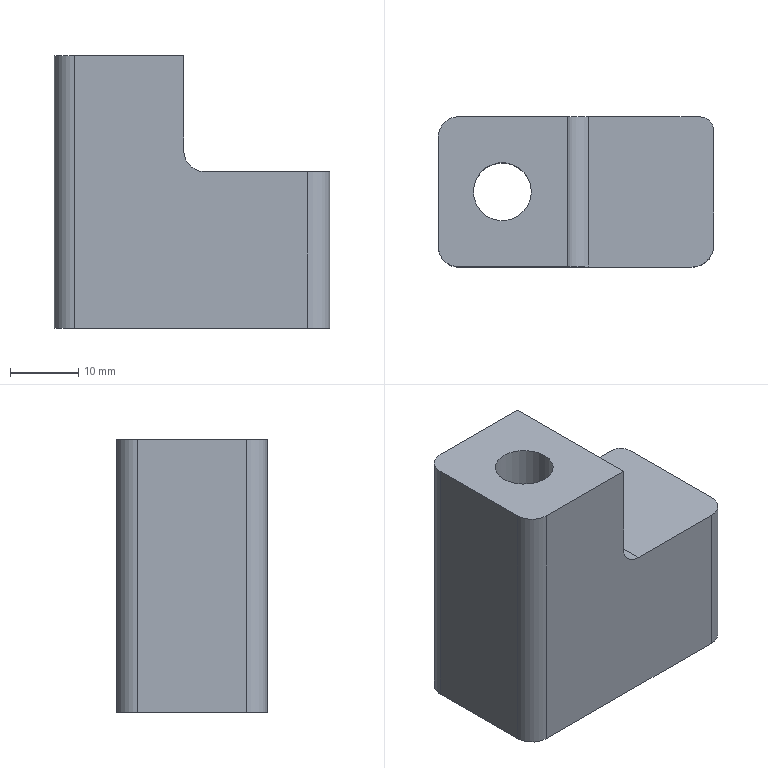Part | NX | features PS-10 2 | 1 solid | 16 faces | box 40.4 x 22 x 40 mm | volume 23471 mm3 | plane 9 | cylinder 7 | commonest cylinder face diameters 6 x3 4 x1 6.4 x1 8.5 x1 14.5 x1
STEP:
#1=CARTESIAN_POINT('',(2525.885,-823.322,883.716));
#2=VERTEX_POINT('',#1);
#3=CARTESIAN_POINT('',(2509.485,-823.322,883.716));
#4=VERTEX_POINT('',#3);
#5=CARTESIAN_POINT('',(-0.000000017,-823.322,883.716));
#6=DIRECTION('',(-1.,0.,0.));
#7=VECTOR('',#6,1000.);
#8=LINE('',#5,#7);
#9=EDGE_CURVE('',#2,#4,#8,.T.);
#10=ORIENTED_EDGE('',*,*,#9,.T.);
#11=CARTESIAN_POINT('',(2509.485,-845.322,883.716));
#12=VERTEX_POINT('',#11);
#13=CARTESIAN_POINT('',(2509.485,0.,883.716));
#14=DIRECTION('',(0.,1.,0.));
#15=VECTOR('',#14,1000.);
#16=LINE('',#13,#15);
#17=EDGE_CURVE('',#4,#12,#16,.F.);
#18=ORIENTED_EDGE('',*,*,#17,.T.);
#19=CARTESIAN_POINT('',(2524.685,-845.322,883.716));
#20=VERTEX_POINT('',#19);
#21=CARTESIAN_POINT('',(0.,-845.322,883.716));
#22=DIRECTION('',(-1.,0.,0.));
#23=VECTOR('',#22,1000.);
#24=LINE('',#21,#23);
#25=EDGE_CURVE('',#20,#12,#24,.T.);
#26=ORIENTED_EDGE('',*,*,#25,.F.);
#27=CARTESIAN_POINT('',(2527.885,-842.122,883.716));
#28=VERTEX_POINT('',#27);
#29=CARTESIAN_POINT('',(2524.685,-842.122,883.716));
#30=DIRECTION('',(0.,0.,1.));
#31=DIRECTION('',(1.,0.,0.));
#32=AXIS2_PLACEMENT_3D('',#29,#30,#31);
#33=CIRCLE('',#32,3.2);
#34=EDGE_CURVE('',#20,#28,#33,.T.);
#35=ORIENTED_EDGE('',*,*,#34,.T.);
#36=CARTESIAN_POINT('',(2527.885,-825.322,883.716));
#37=VERTEX_POINT('',#36);
#38=CARTESIAN_POINT('',(2527.885,0.,883.716));
#39=DIRECTION('',(0.,-1.,0.));
#40=VECTOR('',#39,1000.);
#41=LINE('',#38,#40);
#42=EDGE_CURVE('',#37,#28,#41,.T.);
#43=ORIENTED_EDGE('',*,*,#42,.F.);
#44=CARTESIAN_POINT('',(2525.885,-825.322,883.716));
#45=DIRECTION('',(0.,0.,1.));
#46=DIRECTION('',(1.,0.,0.));
#47=AXIS2_PLACEMENT_3D('',#44,#45,#46);
#48=CIRCLE('',#47,2.);
#49=EDGE_CURVE('',#37,#2,#48,.T.);
#50=ORIENTED_EDGE('',*,*,#49,.T.);
#51=EDGE_LOOP('',(#10,#18,#26,#35,#43,#50));
#52=FACE_BOUND('',#51,.T.);
#53=CARTESIAN_POINT('',(0.,0.,883.716));
#54=DIRECTION('',(0.,0.,1.));
#55=DIRECTION('',(1.,0.,0.));
#56=AXIS2_PLACEMENT_3D('',#53,#54,#55);
#57=PLANE('',#56);
#58=ADVANCED_FACE('',(#52),#57,.T.);
#59=CARTESIAN_POINT('',(2487.485,-842.322,860.716));
#60=VERTEX_POINT('',#59);
#61=CARTESIAN_POINT('',(2487.485,-826.322,860.716));
#62=VERTEX_POINT('',#61);
#63=CARTESIAN_POINT('',(2487.485,0.,860.716));
#64=DIRECTION('',(0.,1.,0.));
#65=VECTOR('',#64,1000.);
#66=LINE('',#63,#65);
#67=EDGE_CURVE('',#60,#62,#66,.T.);
#68=ORIENTED_EDGE('',*,*,#67,.F.);
#69=CARTESIAN_POINT('',(2487.485,-842.322,900.716));
#70=VERTEX_POINT('',#69);
#71=CARTESIAN_POINT('',(2487.485,-842.322,861.517));
#72=DIRECTION('',(0.,0.,1.));
#73=VECTOR('',#72,1000.);
#74=LINE('',#71,#73);
#75=EDGE_CURVE('',#60,#70,#74,.T.);
#76=ORIENTED_EDGE('',*,*,#75,.T.);
#77=CARTESIAN_POINT('',(2487.485,-826.322,900.716));
#78=VERTEX_POINT('',#77);
#79=CARTESIAN_POINT('',(2487.485,-823.072,900.716));
#80=DIRECTION('',(0.,-1.,0.));
#81=VECTOR('',#80,1000.);
#82=LINE('',#79,#81);
#83=EDGE_CURVE('',#78,#70,#82,.T.);
#84=ORIENTED_EDGE('',*,*,#83,.F.);
#85=CARTESIAN_POINT('',(2487.485,-826.322,861.517));
#86=DIRECTION('',(0.,0.,1.));
#87=VECTOR('',#86,1000.);
#88=LINE('',#85,#87);
#89=EDGE_CURVE('',#78,#62,#88,.F.);
#90=ORIENTED_EDGE('',*,*,#89,.T.);
#91=EDGE_LOOP('',(#68,#76,#84,#90));
#92=FACE_BOUND('',#91,.T.);
#93=CARTESIAN_POINT('',(2487.485,-823.072,861.517));
#94=DIRECTION('',(1.,0.,0.));
#95=DIRECTION('',(0.,0.,-1.));
#96=AXIS2_PLACEMENT_3D('',#93,#94,#95);
#97=PLANE('',#96);
#98=ADVANCED_FACE('',(#92),#97,.F.);
#99=ORIENTED_EDGE('',*,*,#25,.T.);
#100=CARTESIAN_POINT('',(2506.485,-845.322,886.716));
#101=VERTEX_POINT('',#100);
#102=CARTESIAN_POINT('',(2509.485,-845.322,886.716));
#103=DIRECTION('',(0.,1.,0.));
#104=DIRECTION('',(0.,0.,1.));
#105=AXIS2_PLACEMENT_3D('',#102,#103,#104);
#106=CIRCLE('',#105,3.);
#107=EDGE_CURVE('',#12,#101,#106,.T.);
#108=ORIENTED_EDGE('',*,*,#107,.T.);
#109=CARTESIAN_POINT('',(2506.485,-845.322,900.716));
#110=VERTEX_POINT('',#109);
#111=CARTESIAN_POINT('',(2506.485,-845.322,900.716));
#112=DIRECTION('',(0.,0.,-1.));
#113=VECTOR('',#112,1000.);
#114=LINE('',#111,#113);
#115=EDGE_CURVE('',#101,#110,#114,.F.);
#116=ORIENTED_EDGE('',*,*,#115,.T.);
#117=CARTESIAN_POINT('',(2490.485,-845.322,900.716));
#118=VERTEX_POINT('',#117);
#119=CARTESIAN_POINT('',(2507.11,-845.322,900.716));
#120=DIRECTION('',(-1.,0.,0.));
#121=VECTOR('',#120,1000.);
#122=LINE('',#119,#121);
#123=EDGE_CURVE('',#110,#118,#122,.T.);
#124=ORIENTED_EDGE('',*,*,#123,.T.);
#125=CARTESIAN_POINT('',(2490.485,-845.322,860.716));
#126=VERTEX_POINT('',#125);
#127=CARTESIAN_POINT('',(2490.485,-845.322,861.517));
#128=DIRECTION('',(0.,0.,1.));
#129=VECTOR('',#128,1000.);
#130=LINE('',#127,#129);
#131=EDGE_CURVE('',#118,#126,#130,.F.);
#132=ORIENTED_EDGE('',*,*,#131,.T.);
#133=CARTESIAN_POINT('',(2524.685,-845.322,860.716));
#134=VERTEX_POINT('',#133);
#135=CARTESIAN_POINT('',(0.,-845.322,860.716));
#136=DIRECTION('',(-1.,0.,0.));
#137=VECTOR('',#136,1000.);
#138=LINE('',#135,#137);
#139=EDGE_CURVE('',#134,#126,#138,.T.);
#140=ORIENTED_EDGE('',*,*,#139,.F.);
#141=CARTESIAN_POINT('',(2524.685,-845.322,861.517));
#142=DIRECTION('',(0.,0.,1.));
#143=VECTOR('',#142,1000.);
#144=LINE('',#141,#143);
#145=EDGE_CURVE('',#134,#20,#144,.T.);
#146=ORIENTED_EDGE('',*,*,#145,.T.);
#147=EDGE_LOOP('',(#99,#108,#116,#124,#132,#140,#146));
#148=FACE_BOUND('',#147,.T.);
#149=CARTESIAN_POINT('',(2507.11,-845.322,861.517));
#150=DIRECTION('',(0.,1.,0.));
#151=DIRECTION('',(0.,0.,1.));
#152=AXIS2_PLACEMENT_3D('',#149,#150,#151);
#153=PLANE('',#152);
#154=ADVANCED_FACE('',(#148),#153,.F.);
#155=ORIENTED_EDGE('',*,*,#34,.F.);
#156=ORIENTED_EDGE('',*,*,#145,.F.);
#157=CARTESIAN_POINT('',(2527.885,-842.122,860.716));
#158=VERTEX_POINT('',#157);
#159=CARTESIAN_POINT('',(2524.685,-842.122,860.716));
#160=DIRECTION('',(0.,0.,1.));
#161=DIRECTION('',(1.,0.,0.));
#162=AXIS2_PLACEMENT_3D('',#159,#160,#161);
#163=CIRCLE('',#162,3.2);
#164=EDGE_CURVE('',#134,#158,#163,.T.);
#165=ORIENTED_EDGE('',*,*,#164,.T.);
#166=CARTESIAN_POINT('',(2527.885,-842.122,861.517));
#167=DIRECTION('',(0.,0.,1.));
#168=VECTOR('',#167,1000.);
#169=LINE('',#166,#168);
#170=EDGE_CURVE('',#158,#28,#169,.T.);
#171=ORIENTED_EDGE('',*,*,#170,.T.);
#172=EDGE_LOOP('',(#155,#156,#165,#171));
#173=FACE_BOUND('',#172,.T.);
#174=CARTESIAN_POINT('',(2524.685,-842.122,861.517));
#175=DIRECTION('',(0.,0.,1.));
#176=DIRECTION('',(1.,0.,0.));
#177=AXIS2_PLACEMENT_3D('',#174,#175,#176);
#178=CYLINDRICAL_SURFACE('',#177,3.2);
#179=ADVANCED_FACE('',(#173),#178,.T.);
#180=CARTESIAN_POINT('',(2527.885,-825.322,860.716));
#181=VERTEX_POINT('',#180);
#182=CARTESIAN_POINT('',(2527.885,0.,860.716));
#183=DIRECTION('',(0.,-1.,0.));
#184=VECTOR('',#183,1000.);
#185=LINE('',#182,#184);
#186=EDGE_CURVE('',#181,#158,#185,.T.);
#187=ORIENTED_EDGE('',*,*,#186,.F.);
#188=CARTESIAN_POINT('',(2527.885,-825.322,872.716));
#189=DIRECTION('',(0.,0.,1.));
#190=VECTOR('',#189,1000.);
#191=LINE('',#188,#190);
#192=EDGE_CURVE('',#181,#37,#191,.T.);
#193=ORIENTED_EDGE('',*,*,#192,.T.);
#194=ORIENTED_EDGE('',*,*,#42,.T.);
#195=ORIENTED_EDGE('',*,*,#170,.F.);
#196=EDGE_LOOP('',(#187,#193,#194,#195));
#197=FACE_BOUND('',#196,.T.);
#198=CARTESIAN_POINT('',(2527.885,-823.122,861.517));
#199=DIRECTION('',(-1.,0.,0.));
#200=DIRECTION('',(0.,0.,1.));
#201=AXIS2_PLACEMENT_3D('',#198,#199,#200);
#202=PLANE('',#201);
#203=ADVANCED_FACE('',(#197),#202,.F.);
#204=ORIENTED_EDGE('',*,*,#9,.F.);
#205=CARTESIAN_POINT('',(2525.885,-823.322,860.716));
#206=VERTEX_POINT('',#205);
#207=CARTESIAN_POINT('',(2525.885,-823.322,860.716));
#208=DIRECTION('',(0.,0.,1.));
#209=VECTOR('',#208,1000.);
#210=LINE('',#207,#209);
#211=EDGE_CURVE('',#2,#206,#210,.F.);
#212=ORIENTED_EDGE('',*,*,#211,.T.);
#213=CARTESIAN_POINT('',(2490.485,-823.322,860.716));
#214=VERTEX_POINT('',#213);
#215=CARTESIAN_POINT('',(-0.000000017,-823.322,860.716));
#216=DIRECTION('',(-1.,0.,0.));
#217=VECTOR('',#216,1000.);
#218=LINE('',#215,#217);
#219=EDGE_CURVE('',#206,#214,#218,.T.);
#220=ORIENTED_EDGE('',*,*,#219,.T.);
#221=CARTESIAN_POINT('',(2490.485,-823.322,900.716));
#222=VERTEX_POINT('',#221);
#223=CARTESIAN_POINT('',(2490.485,-823.322,861.517));
#224=DIRECTION('',(0.,0.,1.));
#225=VECTOR('',#224,1000.);
#226=LINE('',#223,#225);
#227=EDGE_CURVE('',#214,#222,#226,.T.);
#228=ORIENTED_EDGE('',*,*,#227,.T.);
#229=CARTESIAN_POINT('',(2506.485,-823.322,900.716));
#230=VERTEX_POINT('',#229);
#231=CARTESIAN_POINT('',(2656.665,-823.322,900.716));
#232=DIRECTION('',(1.,0.,0.));
#233=VECTOR('',#232,1000.);
#234=LINE('',#231,#233);
#235=EDGE_CURVE('',#222,#230,#234,.T.);
#236=ORIENTED_EDGE('',*,*,#235,.T.);
#237=CARTESIAN_POINT('',(2506.485,-823.322,886.716));
#238=VERTEX_POINT('',#237);
#239=CARTESIAN_POINT('',(2506.485,-823.322,900.716));
#240=DIRECTION('',(0.,0.,-1.));
#241=VECTOR('',#240,1000.);
#242=LINE('',#239,#241);
#243=EDGE_CURVE('',#230,#238,#242,.T.);
#244=ORIENTED_EDGE('',*,*,#243,.T.);
#245=CARTESIAN_POINT('',(2509.485,-823.322,886.716));
#246=DIRECTION('',(0.,1.,0.));
#247=DIRECTION('',(-1.,0.,0.));
#248=AXIS2_PLACEMENT_3D('',#245,#246,#247);
#249=CIRCLE('',#248,3.);
#250=EDGE_CURVE('',#238,#4,#249,.F.);
#251=ORIENTED_EDGE('',*,*,#250,.T.);
#252=EDGE_LOOP('',(#204,#212,#220,#228,#236,#244,#251));
#253=FACE_BOUND('',#252,.T.);
#254=CARTESIAN_POINT('',(2656.665,-823.322,861.517));
#255=DIRECTION('',(0.,1.,0.));
#256=DIRECTION('',(-1.,0.,0.));
#257=AXIS2_PLACEMENT_3D('',#254,#255,#256);
#258=PLANE('',#257);
#259=ADVANCED_FACE('',(#253),#258,.T.);
#260=CARTESIAN_POINT('',(2504.135,-834.322,860.716));
#261=VERTEX_POINT('',#260);
#262=CARTESIAN_POINT('',(2496.885,-834.322,860.716));
#263=DIRECTION('',(0.,0.,1.));
#264=DIRECTION('',(1.,0.,0.));
#265=AXIS2_PLACEMENT_3D('',#262,#263,#264);
#266=CIRCLE('',#265,7.25);
#267=EDGE_CURVE('',#261,#261,#266,.T.);
#268=ORIENTED_EDGE('',*,*,#267,.T.);
#269=EDGE_LOOP('',(#268));
#270=FACE_BOUND('',#269,.T.);
#271=ORIENTED_EDGE('',*,*,#219,.F.);
#272=CARTESIAN_POINT('',(2525.885,-825.322,860.716));
#273=DIRECTION('',(0.,0.,1.));
#274=DIRECTION('',(1.,0.,0.));
#275=AXIS2_PLACEMENT_3D('',#272,#273,#274);
#276=CIRCLE('',#275,2.);
#277=EDGE_CURVE('',#206,#181,#276,.F.);
#278=ORIENTED_EDGE('',*,*,#277,.T.);
#279=ORIENTED_EDGE('',*,*,#186,.T.);
#280=ORIENTED_EDGE('',*,*,#164,.F.);
#281=ORIENTED_EDGE('',*,*,#139,.T.);
#282=CARTESIAN_POINT('',(2490.485,-842.322,860.716));
#283=DIRECTION('',(0.,0.,1.));
#284=DIRECTION('',(1.,0.,0.));
#285=AXIS2_PLACEMENT_3D('',#282,#283,#284);
#286=CIRCLE('',#285,3.);
#287=EDGE_CURVE('',#126,#60,#286,.F.);
#288=ORIENTED_EDGE('',*,*,#287,.T.);
#289=ORIENTED_EDGE('',*,*,#67,.T.);
#290=CARTESIAN_POINT('',(2490.485,-826.322,860.716));
#291=DIRECTION('',(0.,0.,1.));
#292=DIRECTION('',(1.,0.,0.));
#293=AXIS2_PLACEMENT_3D('',#290,#291,#292);
#294=CIRCLE('',#293,3.);
#295=EDGE_CURVE('',#62,#214,#294,.F.);
#296=ORIENTED_EDGE('',*,*,#295,.T.);
#297=EDGE_LOOP('',(#271,#278,#279,#280,#281,#288,#289,#296));
#298=FACE_BOUND('',#297,.T.);
#299=CARTESIAN_POINT('',(0.,0.,860.716));
#300=DIRECTION('',(0.,0.,1.));
#301=DIRECTION('',(1.,0.,0.));
#302=AXIS2_PLACEMENT_3D('',#299,#300,#301);
#303=PLANE('',#302);
#304=ADVANCED_FACE('',(#270,#298),#303,.F.);
#305=ORIENTED_EDGE('',*,*,#287,.F.);
#306=ORIENTED_EDGE('',*,*,#131,.F.);
#307=CARTESIAN_POINT('',(2490.485,-842.322,900.716));
#308=DIRECTION('',(0.,0.,1.));
#309=DIRECTION('',(1.,0.,0.));
#310=AXIS2_PLACEMENT_3D('',#307,#308,#309);
#311=CIRCLE('',#310,3.);
#312=EDGE_CURVE('',#118,#70,#311,.F.);
#313=ORIENTED_EDGE('',*,*,#312,.T.);
#314=ORIENTED_EDGE('',*,*,#75,.F.);
#315=EDGE_LOOP('',(#305,#306,#313,#314));
#316=FACE_BOUND('',#315,.T.);
#317=CARTESIAN_POINT('',(2490.485,-842.322,861.517));
#318=DIRECTION('',(0.,0.,1.));
#319=DIRECTION('',(1.,0.,0.));
#320=AXIS2_PLACEMENT_3D('',#317,#318,#319);
#321=CYLINDRICAL_SURFACE('',#320,3.);
#322=ADVANCED_FACE('',(#316),#321,.T.);
#323=ORIENTED_EDGE('',*,*,#295,.F.);
#324=ORIENTED_EDGE('',*,*,#89,.F.);
#325=CARTESIAN_POINT('',(2490.485,-826.322,900.716));
#326=DIRECTION('',(0.,0.,1.));
#327=DIRECTION('',(1.,0.,0.));
#328=AXIS2_PLACEMENT_3D('',#325,#326,#327);
#329=CIRCLE('',#328,3.);
#330=EDGE_CURVE('',#78,#222,#329,.F.);
#331=ORIENTED_EDGE('',*,*,#330,.T.);
#332=ORIENTED_EDGE('',*,*,#227,.F.);
#333=EDGE_LOOP('',(#323,#324,#331,#332));
#334=FACE_BOUND('',#333,.T.);
#335=CARTESIAN_POINT('',(2490.485,-826.322,861.517));
#336=DIRECTION('',(0.,0.,-1.));
#337=DIRECTION('',(-1.,0.,0.));
#338=AXIS2_PLACEMENT_3D('',#335,#336,#337);
#339=CYLINDRICAL_SURFACE('',#338,3.);
#340=ADVANCED_FACE('',(#334),#339,.T.);
#341=ORIENTED_EDGE('',*,*,#277,.F.);
#342=ORIENTED_EDGE('',*,*,#211,.F.);
#343=ORIENTED_EDGE('',*,*,#49,.F.);
#344=ORIENTED_EDGE('',*,*,#192,.F.);
#345=EDGE_LOOP('',(#341,#342,#343,#344));
#346=FACE_BOUND('',#345,.T.);
#347=CARTESIAN_POINT('',(2525.885,-825.322,861.517));
#348=DIRECTION('',(0.,0.,-1.));
#349=DIRECTION('',(-1.,0.,0.));
#350=AXIS2_PLACEMENT_3D('',#347,#348,#349);
#351=CYLINDRICAL_SURFACE('',#350,2.);
#352=ADVANCED_FACE('',(#346),#351,.T.);
#353=ORIENTED_EDGE('',*,*,#115,.F.);
#354=CARTESIAN_POINT('',(2506.485,-823.072,886.716));
#355=DIRECTION('',(0.,1.,0.));
#356=VECTOR('',#355,1000.);
#357=LINE('',#354,#356);
#358=EDGE_CURVE('',#101,#238,#357,.T.);
#359=ORIENTED_EDGE('',*,*,#358,.T.);
#360=ORIENTED_EDGE('',*,*,#243,.F.);
#361=CARTESIAN_POINT('',(2506.485,-823.072,900.716));
#362=DIRECTION('',(0.,1.,0.));
#363=VECTOR('',#362,1000.);
#364=LINE('',#361,#363);
#365=EDGE_CURVE('',#110,#230,#364,.T.);
#366=ORIENTED_EDGE('',*,*,#365,.F.);
#367=EDGE_LOOP('',(#353,#359,#360,#366));
#368=FACE_BOUND('',#367,.T.);
#369=CARTESIAN_POINT('',(2506.485,-823.072,900.716));
#370=DIRECTION('',(-1.,0.,0.));
#371=DIRECTION('',(0.,0.,1.));
#372=AXIS2_PLACEMENT_3D('',#369,#370,#371);
#373=PLANE('',#372);
#374=ADVANCED_FACE('',(#368),#373,.F.);
#375=CARTESIAN_POINT('',(2501.135,-834.322,900.716));
#376=VERTEX_POINT('',#375);
#377=CARTESIAN_POINT('',(2496.885,-834.322,900.716));
#378=DIRECTION('',(0.,0.,1.));
#379=DIRECTION('',(1.,0.,0.));
#380=AXIS2_PLACEMENT_3D('',#377,#378,#379);
#381=CIRCLE('',#380,4.25);
#382=EDGE_CURVE('',#376,#376,#381,.T.);
#383=ORIENTED_EDGE('',*,*,#382,.F.);
#384=EDGE_LOOP('',(#383));
#385=FACE_BOUND('',#384,.T.);
#386=ORIENTED_EDGE('',*,*,#123,.F.);
#387=ORIENTED_EDGE('',*,*,#365,.T.);
#388=ORIENTED_EDGE('',*,*,#235,.F.);
#389=ORIENTED_EDGE('',*,*,#330,.F.);
#390=ORIENTED_EDGE('',*,*,#83,.T.);
#391=ORIENTED_EDGE('',*,*,#312,.F.);
#392=EDGE_LOOP('',(#386,#387,#388,#389,#390,#391));
#393=FACE_BOUND('',#392,.T.);
#394=CARTESIAN_POINT('',(0.,0.,900.716));
#395=DIRECTION('',(0.,0.,1.));
#396=DIRECTION('',(1.,0.,0.));
#397=AXIS2_PLACEMENT_3D('',#394,#395,#396);
#398=PLANE('',#397);
#399=ADVANCED_FACE('',(#385,#393),#398,.T.);
#400=ORIENTED_EDGE('',*,*,#107,.F.);
#401=ORIENTED_EDGE('',*,*,#17,.F.);
#402=ORIENTED_EDGE('',*,*,#250,.F.);
#403=ORIENTED_EDGE('',*,*,#358,.F.);
#404=EDGE_LOOP('',(#400,#401,#402,#403));
#405=FACE_BOUND('',#404,.T.);
#406=CARTESIAN_POINT('',(2509.485,-823.072,886.716));
#407=DIRECTION('',(0.,1.,0.));
#408=DIRECTION('',(0.,0.,1.));
#409=AXIS2_PLACEMENT_3D('',#406,#407,#408);
#410=CYLINDRICAL_SURFACE('',#409,3.);
#411=ADVANCED_FACE('',(#405),#410,.F.);
#412=CARTESIAN_POINT('',(2489.635,-834.322,875.716));
#413=VERTEX_POINT('',#412);
#414=CARTESIAN_POINT('',(2496.885,-834.322,875.716));
#415=DIRECTION('',(0.,0.,-1.));
#416=DIRECTION('',(-1.,0.,0.));
#417=AXIS2_PLACEMENT_3D('',#414,#415,#416);
#418=CIRCLE('',#417,7.25);
#419=EDGE_CURVE('',#413,#413,#418,.F.);
#420=ORIENTED_EDGE('',*,*,#419,.T.);
#421=EDGE_LOOP('',(#420));
#422=FACE_BOUND('',#421,.T.);
#423=ORIENTED_EDGE('',*,*,#267,.F.);
#424=EDGE_LOOP('',(#423));
#425=FACE_BOUND('',#424,.T.);
#426=CARTESIAN_POINT('',(2496.885,-834.322,875.716));
#427=DIRECTION('',(0.,0.,-1.));
#428=DIRECTION('',(-1.,0.,0.));
#429=AXIS2_PLACEMENT_3D('',#426,#427,#428);
#430=CYLINDRICAL_SURFACE('',#429,7.25);
#431=ADVANCED_FACE('',(#422,#425),#430,.F.);
#432=ORIENTED_EDGE('',*,*,#382,.T.);
#433=EDGE_LOOP('',(#432));
#434=FACE_BOUND('',#433,.T.);
#435=CARTESIAN_POINT('',(2492.635,-834.322,875.716));
#436=VERTEX_POINT('',#435);
#437=CARTESIAN_POINT('',(2496.885,-834.322,875.716));
#438=DIRECTION('',(0.,0.,-1.));
#439=DIRECTION('',(-1.,0.,0.));
#440=AXIS2_PLACEMENT_3D('',#437,#438,#439);
#441=CIRCLE('',#440,4.25);
#442=EDGE_CURVE('',#436,#436,#441,.T.);
#443=ORIENTED_EDGE('',*,*,#442,.T.);
#444=EDGE_LOOP('',(#443));
#445=FACE_BOUND('',#444,.T.);
#446=CARTESIAN_POINT('',(2496.885,-834.322,901.716));
#447=DIRECTION('',(0.,0.,-1.));
#448=DIRECTION('',(-1.,0.,0.));
#449=AXIS2_PLACEMENT_3D('',#446,#447,#448);
#450=CYLINDRICAL_SURFACE('',#449,4.25);
#451=ADVANCED_FACE('',(#434,#445),#450,.F.);
#452=ORIENTED_EDGE('',*,*,#442,.F.);
#453=EDGE_LOOP('',(#452));
#454=FACE_BOUND('',#453,.T.);
#455=ORIENTED_EDGE('',*,*,#419,.F.);
#456=EDGE_LOOP('',(#455));
#457=FACE_BOUND('',#456,.T.);
#458=CARTESIAN_POINT('',(2496.885,-834.322,875.716));
#459=DIRECTION('',(0.,0.,-1.));
#460=DIRECTION('',(-1.,0.,0.));
#461=AXIS2_PLACEMENT_3D('',#458,#459,#460);
#462=PLANE('',#461);
#463=ADVANCED_FACE('',(#454,#457),#462,.T.);
#464=CLOSED_SHELL('',(#58,#98,#154,#179,#203,#259,#304,#322,#340,#352,#374,#399,#411,#431,#451,#463));
#465=MANIFOLD_SOLID_BREP('',#464);
#466=(LENGTH_UNIT()NAMED_UNIT(*)SI_UNIT(.MILLI.,.METRE.));
#467=UNCERTAINTY_MEASURE_WITH_UNIT(LENGTH_MEASURE(0.00001),#466,'','');
#468=(NAMED_UNIT(*)PLANE_ANGLE_UNIT()SI_UNIT($,.RADIAN.));
#469=(NAMED_UNIT(*)SI_UNIT($,.STERADIAN.)SOLID_ANGLE_UNIT());
#470=(GEOMETRIC_REPRESENTATION_CONTEXT(3)GLOBAL_UNCERTAINTY_ASSIGNED_CONTEXT((#467))GLOBAL_UNIT_ASSIGNED_CONTEXT((#466,#468,#469))REPRESENTATION_CONTEXT('',''));
#471=ADVANCED_BREP_SHAPE_REPRESENTATION('',(#465),#470);